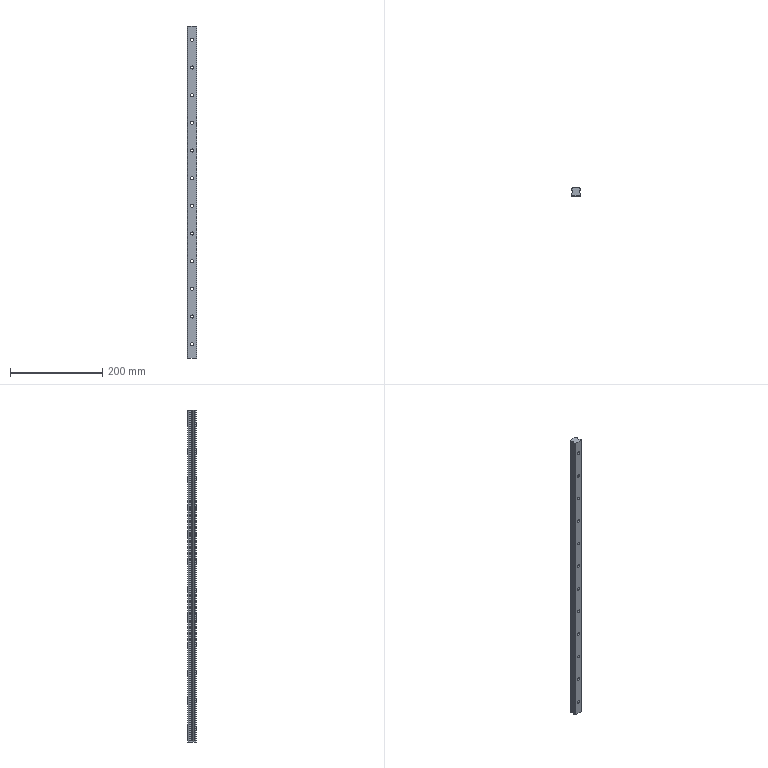Part | STEP file | HGR20_3_AF0_1-700 | 1 solid | 104 faces | box 20 x 17.5 x 720 mm | volume 203064 mm3 | cylinder 70 | plane 34 | commonest cylinder face diameters 6.6 x24 11 x24 1 x12 2 x6 4.06 x4